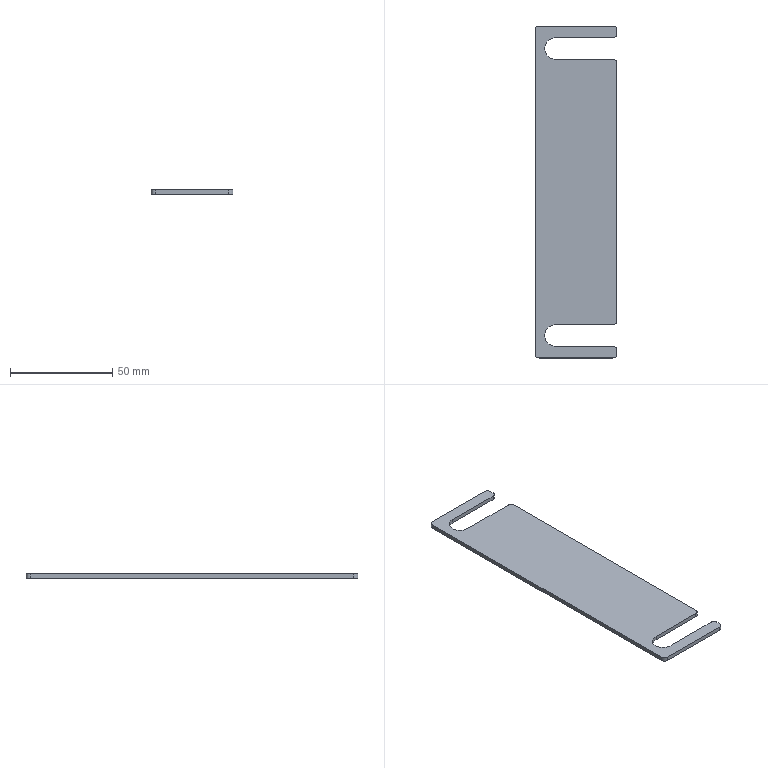Part | SolidWorks | features ICE 2, Extrusion 1, Fillet 1 | 1 solid | 22 faces | box 40 x 162 x 2 mm | volume 11517 mm3 | plane 12 | cylinder 10 | commonest cylinder face diameters 4 x8 10.5 x2
STEP:
#1=CARTESIAN_POINT('',(20.,77.25,2.));
#2=VERTEX_POINT('',#1);
#3=CARTESIAN_POINT('',(20.,79.,2.));
#4=VERTEX_POINT('',#3);
#5=CARTESIAN_POINT('',(20.,-81.,2.));
#6=DIRECTION('',(0.,1.,0.));
#7=VECTOR('',#6,1000.);
#8=LINE('',#5,#7);
#9=EDGE_CURVE('',#2,#4,#8,.T.);
#10=ORIENTED_EDGE('',*,*,#9,.F.);
#11=CARTESIAN_POINT('',(20.,77.25,0.));
#12=VERTEX_POINT('',#11);
#13=CARTESIAN_POINT('',(20.,77.25,2.));
#14=DIRECTION('',(0.,0.,-1.));
#15=VECTOR('',#14,1000.);
#16=LINE('',#13,#15);
#17=EDGE_CURVE('',#2,#12,#16,.T.);
#18=ORIENTED_EDGE('',*,*,#17,.T.);
#19=CARTESIAN_POINT('',(20.,79.,0.));
#20=VERTEX_POINT('',#19);
#21=CARTESIAN_POINT('',(20.,-81.,0.));
#22=DIRECTION('',(0.,1.,0.));
#23=VECTOR('',#22,1000.);
#24=LINE('',#21,#23);
#25=EDGE_CURVE('',#12,#20,#24,.T.);
#26=ORIENTED_EDGE('',*,*,#25,.T.);
#27=CARTESIAN_POINT('',(20.,79.,2.));
#28=DIRECTION('',(0.,0.,1.));
#29=VECTOR('',#28,1000.);
#30=LINE('',#27,#29);
#31=EDGE_CURVE('',#20,#4,#30,.T.);
#32=ORIENTED_EDGE('',*,*,#31,.T.);
#33=EDGE_LOOP('',(#10,#18,#26,#32));
#34=FACE_OUTER_BOUND('',#33,.T.);
#35=CARTESIAN_POINT('',(20.,-81.,2.));
#36=DIRECTION('',(-1.,0.,0.));
#37=DIRECTION('',(0.,0.,1.));
#38=AXIS2_PLACEMENT_3D('',#35,#36,#37);
#39=PLANE('',#38);
#40=ADVANCED_FACE('',(#34),#39,.F.);
#41=CARTESIAN_POINT('',(20.,-62.781,2.));
#42=VERTEX_POINT('',#41);
#43=CARTESIAN_POINT('',(20.,62.75,2.));
#44=VERTEX_POINT('',#43);
#45=CARTESIAN_POINT('',(20.,-81.,2.));
#46=DIRECTION('',(0.,1.,0.));
#47=VECTOR('',#46,1000.);
#48=LINE('',#45,#47);
#49=EDGE_CURVE('',#42,#44,#48,.T.);
#50=ORIENTED_EDGE('',*,*,#49,.F.);
#51=CARTESIAN_POINT('',(20.,-62.781,0.));
#52=VERTEX_POINT('',#51);
#53=CARTESIAN_POINT('',(20.,-62.781,2.));
#54=DIRECTION('',(0.,0.,-1.));
#55=VECTOR('',#54,1000.);
#56=LINE('',#53,#55);
#57=EDGE_CURVE('',#42,#52,#56,.T.);
#58=ORIENTED_EDGE('',*,*,#57,.T.);
#59=CARTESIAN_POINT('',(20.,62.75,0.));
#60=VERTEX_POINT('',#59);
#61=CARTESIAN_POINT('',(20.,-81.,0.));
#62=DIRECTION('',(0.,1.,0.));
#63=VECTOR('',#62,1000.);
#64=LINE('',#61,#63);
#65=EDGE_CURVE('',#52,#60,#64,.T.);
#66=ORIENTED_EDGE('',*,*,#65,.T.);
#67=CARTESIAN_POINT('',(20.,62.75,2.));
#68=DIRECTION('',(0.,0.,1.));
#69=VECTOR('',#68,1000.);
#70=LINE('',#67,#69);
#71=EDGE_CURVE('',#60,#44,#70,.T.);
#72=ORIENTED_EDGE('',*,*,#71,.T.);
#73=EDGE_LOOP('',(#50,#58,#66,#72));
#74=FACE_OUTER_BOUND('',#73,.T.);
#75=CARTESIAN_POINT('',(20.,-81.,2.));
#76=DIRECTION('',(-1.,0.,0.));
#77=DIRECTION('',(0.,0.,1.));
#78=AXIS2_PLACEMENT_3D('',#75,#76,#77);
#79=PLANE('',#78);
#80=ADVANCED_FACE('',(#74),#79,.F.);
#81=CARTESIAN_POINT('',(-10.,75.25,2.));
#82=VERTEX_POINT('',#81);
#83=CARTESIAN_POINT('',(-10.,75.25,0.));
#84=VERTEX_POINT('',#83);
#85=CARTESIAN_POINT('',(-10.,75.25,-1.));
#86=DIRECTION('',(0.,0.,-1.));
#87=VECTOR('',#86,1000.);
#88=LINE('',#85,#87);
#89=EDGE_CURVE('',#82,#84,#88,.T.);
#90=ORIENTED_EDGE('',*,*,#89,.F.);
#91=CARTESIAN_POINT('',(-10.,64.75,2.));
#92=VERTEX_POINT('',#91);
#93=CARTESIAN_POINT('',(-10.,70.,2.));
#94=DIRECTION('',(0.,0.,1.));
#95=DIRECTION('',(1.,0.,0.));
#96=AXIS2_PLACEMENT_3D('',#93,#94,#95);
#97=CIRCLE('',#96,5.25);
#98=EDGE_CURVE('',#82,#92,#97,.T.);
#99=ORIENTED_EDGE('',*,*,#98,.T.);
#100=CARTESIAN_POINT('',(-10.,64.75,0.));
#101=VERTEX_POINT('',#100);
#102=CARTESIAN_POINT('',(-10.,64.75,-1.));
#103=DIRECTION('',(0.,0.,-1.));
#104=VECTOR('',#103,1000.);
#105=LINE('',#102,#104);
#106=EDGE_CURVE('',#92,#101,#105,.T.);
#107=ORIENTED_EDGE('',*,*,#106,.T.);
#108=CARTESIAN_POINT('',(-10.,70.,0.));
#109=DIRECTION('',(0.,0.,1.));
#110=DIRECTION('',(1.,0.,0.));
#111=AXIS2_PLACEMENT_3D('',#108,#109,#110);
#112=CIRCLE('',#111,5.25);
#113=EDGE_CURVE('',#84,#101,#112,.T.);
#114=ORIENTED_EDGE('',*,*,#113,.F.);
#115=EDGE_LOOP('',(#90,#99,#107,#114));
#116=FACE_OUTER_BOUND('',#115,.T.);
#117=CARTESIAN_POINT('',(-10.,70.,-1.));
#118=DIRECTION('',(0.,0.,1.));
#119=DIRECTION('',(1.,0.,0.));
#120=AXIS2_PLACEMENT_3D('',#117,#118,#119);
#121=CYLINDRICAL_SURFACE('',#120,5.25);
#122=ADVANCED_FACE('',(#116),#121,.F.);
#123=CARTESIAN_POINT('',(-20.,79.,0.));
#124=VERTEX_POINT('',#123);
#125=CARTESIAN_POINT('',(-20.,-79.,0.));
#126=VERTEX_POINT('',#125);
#127=CARTESIAN_POINT('',(-20.,-81.,0.));
#128=DIRECTION('',(0.,-1.,0.));
#129=VECTOR('',#128,1000.);
#130=LINE('',#127,#129);
#131=EDGE_CURVE('',#124,#126,#130,.T.);
#132=ORIENTED_EDGE('',*,*,#131,.T.);
#133=CARTESIAN_POINT('',(-20.,-79.,2.));
#134=VERTEX_POINT('',#133);
#135=CARTESIAN_POINT('',(-20.,-79.,2.));
#136=DIRECTION('',(0.,0.,1.));
#137=VECTOR('',#136,1000.);
#138=LINE('',#135,#137);
#139=EDGE_CURVE('',#126,#134,#138,.T.);
#140=ORIENTED_EDGE('',*,*,#139,.T.);
#141=CARTESIAN_POINT('',(-20.,79.,2.));
#142=VERTEX_POINT('',#141);
#143=CARTESIAN_POINT('',(-20.,-81.,2.));
#144=DIRECTION('',(0.,-1.,0.));
#145=VECTOR('',#144,1000.);
#146=LINE('',#143,#145);
#147=EDGE_CURVE('',#142,#134,#146,.T.);
#148=ORIENTED_EDGE('',*,*,#147,.F.);
#149=CARTESIAN_POINT('',(-20.,79.,2.));
#150=DIRECTION('',(0.,0.,-1.));
#151=VECTOR('',#150,1000.);
#152=LINE('',#149,#151);
#153=EDGE_CURVE('',#142,#124,#152,.T.);
#154=ORIENTED_EDGE('',*,*,#153,.T.);
#155=EDGE_LOOP('',(#132,#140,#148,#154));
#156=FACE_OUTER_BOUND('',#155,.T.);
#157=CARTESIAN_POINT('',(-20.,-81.,2.));
#158=DIRECTION('',(1.,0.,0.));
#159=DIRECTION('',(0.,0.,-1.));
#160=AXIS2_PLACEMENT_3D('',#157,#158,#159);
#161=PLANE('',#160);
#162=ADVANCED_FACE('',(#156),#161,.F.);
#163=CARTESIAN_POINT('',(-18.,-81.,2.));
#164=VERTEX_POINT('',#163);
#165=CARTESIAN_POINT('',(18.,-81.,2.));
#166=VERTEX_POINT('',#165);
#167=CARTESIAN_POINT('',(20.,-81.,2.));
#168=DIRECTION('',(1.,0.,0.));
#169=VECTOR('',#168,1000.);
#170=LINE('',#167,#169);
#171=EDGE_CURVE('',#164,#166,#170,.T.);
#172=ORIENTED_EDGE('',*,*,#171,.F.);
#173=CARTESIAN_POINT('',(-18.,-81.,0.));
#174=VERTEX_POINT('',#173);
#175=CARTESIAN_POINT('',(-18.,-81.,2.));
#176=DIRECTION('',(0.,0.,-1.));
#177=VECTOR('',#176,1000.);
#178=LINE('',#175,#177);
#179=EDGE_CURVE('',#164,#174,#178,.T.);
#180=ORIENTED_EDGE('',*,*,#179,.T.);
#181=CARTESIAN_POINT('',(18.,-81.,0.));
#182=VERTEX_POINT('',#181);
#183=CARTESIAN_POINT('',(20.,-81.,0.));
#184=DIRECTION('',(1.,0.,0.));
#185=VECTOR('',#184,1000.);
#186=LINE('',#183,#185);
#187=EDGE_CURVE('',#174,#182,#186,.T.);
#188=ORIENTED_EDGE('',*,*,#187,.T.);
#189=CARTESIAN_POINT('',(18.,-81.,2.));
#190=DIRECTION('',(0.,0.,1.));
#191=VECTOR('',#190,1000.);
#192=LINE('',#189,#191);
#193=EDGE_CURVE('',#182,#166,#192,.T.);
#194=ORIENTED_EDGE('',*,*,#193,.T.);
#195=EDGE_LOOP('',(#172,#180,#188,#194));
#196=FACE_OUTER_BOUND('',#195,.T.);
#197=CARTESIAN_POINT('',(20.,-81.,2.));
#198=DIRECTION('',(0.,1.,0.));
#199=DIRECTION('',(0.,0.,1.));
#200=AXIS2_PLACEMENT_3D('',#197,#198,#199);
#201=PLANE('',#200);
#202=ADVANCED_FACE('',(#196),#201,.F.);
#203=CARTESIAN_POINT('',(20.,-79.,0.));
#204=VERTEX_POINT('',#203);
#205=CARTESIAN_POINT('',(20.,-77.219,0.));
#206=VERTEX_POINT('',#205);
#207=CARTESIAN_POINT('',(20.,-81.,0.));
#208=DIRECTION('',(0.,1.,0.));
#209=VECTOR('',#208,1000.);
#210=LINE('',#207,#209);
#211=EDGE_CURVE('',#204,#206,#210,.T.);
#212=ORIENTED_EDGE('',*,*,#211,.T.);
#213=CARTESIAN_POINT('',(20.,-77.219,2.));
#214=VERTEX_POINT('',#213);
#215=CARTESIAN_POINT('',(20.,-77.219,2.));
#216=DIRECTION('',(0.,0.,1.));
#217=VECTOR('',#216,1000.);
#218=LINE('',#215,#217);
#219=EDGE_CURVE('',#206,#214,#218,.T.);
#220=ORIENTED_EDGE('',*,*,#219,.T.);
#221=CARTESIAN_POINT('',(20.,-79.,2.));
#222=VERTEX_POINT('',#221);
#223=CARTESIAN_POINT('',(20.,-81.,2.));
#224=DIRECTION('',(0.,1.,0.));
#225=VECTOR('',#224,1000.);
#226=LINE('',#223,#225);
#227=EDGE_CURVE('',#222,#214,#226,.T.);
#228=ORIENTED_EDGE('',*,*,#227,.F.);
#229=CARTESIAN_POINT('',(20.,-79.,2.));
#230=DIRECTION('',(0.,0.,-1.));
#231=VECTOR('',#230,1000.);
#232=LINE('',#229,#231);
#233=EDGE_CURVE('',#222,#204,#232,.T.);
#234=ORIENTED_EDGE('',*,*,#233,.T.);
#235=EDGE_LOOP('',(#212,#220,#228,#234));
#236=FACE_OUTER_BOUND('',#235,.T.);
#237=CARTESIAN_POINT('',(20.,-81.,2.));
#238=DIRECTION('',(-1.,0.,0.));
#239=DIRECTION('',(0.,0.,1.));
#240=AXIS2_PLACEMENT_3D('',#237,#238,#239);
#241=PLANE('',#240);
#242=ADVANCED_FACE('',(#236),#241,.F.);
#243=CARTESIAN_POINT('',(18.,81.,0.));
#244=VERTEX_POINT('',#243);
#245=CARTESIAN_POINT('',(-18.,81.,0.));
#246=VERTEX_POINT('',#245);
#247=CARTESIAN_POINT('',(20.,81.,0.));
#248=DIRECTION('',(-1.,0.,0.));
#249=VECTOR('',#248,1000.);
#250=LINE('',#247,#249);
#251=EDGE_CURVE('',#244,#246,#250,.T.);
#252=ORIENTED_EDGE('',*,*,#251,.T.);
#253=CARTESIAN_POINT('',(-18.,81.,2.));
#254=VERTEX_POINT('',#253);
#255=CARTESIAN_POINT('',(-18.,81.,2.));
#256=DIRECTION('',(0.,0.,1.));
#257=VECTOR('',#256,1000.);
#258=LINE('',#255,#257);
#259=EDGE_CURVE('',#246,#254,#258,.T.);
#260=ORIENTED_EDGE('',*,*,#259,.T.);
#261=CARTESIAN_POINT('',(18.,81.,2.));
#262=VERTEX_POINT('',#261);
#263=CARTESIAN_POINT('',(20.,81.,2.));
#264=DIRECTION('',(-1.,0.,0.));
#265=VECTOR('',#264,1000.);
#266=LINE('',#263,#265);
#267=EDGE_CURVE('',#262,#254,#266,.T.);
#268=ORIENTED_EDGE('',*,*,#267,.F.);
#269=CARTESIAN_POINT('',(18.,81.,2.));
#270=DIRECTION('',(0.,0.,-1.));
#271=VECTOR('',#270,1000.);
#272=LINE('',#269,#271);
#273=EDGE_CURVE('',#262,#244,#272,.T.);
#274=ORIENTED_EDGE('',*,*,#273,.T.);
#275=EDGE_LOOP('',(#252,#260,#268,#274));
#276=FACE_OUTER_BOUND('',#275,.T.);
#277=CARTESIAN_POINT('',(20.,81.,2.));
#278=DIRECTION('',(0.,-1.,0.));
#279=DIRECTION('',(0.,0.,-1.));
#280=AXIS2_PLACEMENT_3D('',#277,#278,#279);
#281=PLANE('',#280);
#282=ADVANCED_FACE('',(#276),#281,.F.);
#283=ORIENTED_EDGE('',*,*,#227,.T.);
#284=CARTESIAN_POINT('',(18.,-75.219,2.));
#285=VERTEX_POINT('',#284);
#286=CARTESIAN_POINT('',(18.,-77.219,2.));
#287=DIRECTION('',(0.,0.,1.));
#288=DIRECTION('',(1.,0.,0.));
#289=AXIS2_PLACEMENT_3D('',#286,#287,#288);
#290=CIRCLE('',#289,2.);
#291=EDGE_CURVE('',#214,#285,#290,.T.);
#292=ORIENTED_EDGE('',*,*,#291,.T.);
#293=CARTESIAN_POINT('',(-9.434,-75.219,2.));
#294=VERTEX_POINT('',#293);
#295=CARTESIAN_POINT('',(-9.434,-75.219,2.));
#296=DIRECTION('',(1.,0.,0.));
#297=VECTOR('',#296,1000.);
#298=LINE('',#295,#297);
#299=EDGE_CURVE('',#294,#285,#298,.T.);
#300=ORIENTED_EDGE('',*,*,#299,.F.);
#301=CARTESIAN_POINT('',(-9.434,-64.781,2.));
#302=VERTEX_POINT('',#301);
#303=CARTESIAN_POINT('',(-10.,-70.,2.));
#304=DIRECTION('',(0.,0.,1.));
#305=DIRECTION('',(1.,0.,0.));
#306=AXIS2_PLACEMENT_3D('',#303,#304,#305);
#307=CIRCLE('',#306,5.25);
#308=EDGE_CURVE('',#302,#294,#307,.T.);
#309=ORIENTED_EDGE('',*,*,#308,.F.);
#310=CARTESIAN_POINT('',(18.,-64.781,2.));
#311=VERTEX_POINT('',#310);
#312=CARTESIAN_POINT('',(-9.434,-64.781,2.));
#313=DIRECTION('',(-1.,0.,0.));
#314=VECTOR('',#313,1000.);
#315=LINE('',#312,#314);
#316=EDGE_CURVE('',#311,#302,#315,.T.);
#317=ORIENTED_EDGE('',*,*,#316,.F.);
#318=CARTESIAN_POINT('',(18.,-62.781,2.));
#319=DIRECTION('',(0.,0.,1.));
#320=DIRECTION('',(1.,0.,0.));
#321=AXIS2_PLACEMENT_3D('',#318,#319,#320);
#322=CIRCLE('',#321,2.);
#323=EDGE_CURVE('',#311,#42,#322,.T.);
#324=ORIENTED_EDGE('',*,*,#323,.T.);
#325=ORIENTED_EDGE('',*,*,#49,.T.);
#326=CARTESIAN_POINT('',(18.,64.75,2.));
#327=VERTEX_POINT('',#326);
#328=CARTESIAN_POINT('',(18.,62.75,2.));
#329=DIRECTION('',(0.,0.,1.));
#330=DIRECTION('',(1.,0.,0.));
#331=AXIS2_PLACEMENT_3D('',#328,#329,#330);
#332=CIRCLE('',#331,2.);
#333=EDGE_CURVE('',#44,#327,#332,.T.);
#334=ORIENTED_EDGE('',*,*,#333,.T.);
#335=CARTESIAN_POINT('',(-10.,64.75,2.));
#336=DIRECTION('',(1.,0.,0.));
#337=VECTOR('',#336,1000.);
#338=LINE('',#335,#337);
#339=EDGE_CURVE('',#92,#327,#338,.T.);
#340=ORIENTED_EDGE('',*,*,#339,.F.);
#341=ORIENTED_EDGE('',*,*,#98,.F.);
#342=CARTESIAN_POINT('',(18.,75.25,2.));
#343=VERTEX_POINT('',#342);
#344=CARTESIAN_POINT('',(-10.,75.25,2.));
#345=DIRECTION('',(-1.,0.,0.));
#346=VECTOR('',#345,1000.);
#347=LINE('',#344,#346);
#348=EDGE_CURVE('',#343,#82,#347,.T.);
#349=ORIENTED_EDGE('',*,*,#348,.F.);
#350=CARTESIAN_POINT('',(18.,77.25,2.));
#351=DIRECTION('',(0.,0.,1.));
#352=DIRECTION('',(1.,0.,0.));
#353=AXIS2_PLACEMENT_3D('',#350,#351,#352);
#354=CIRCLE('',#353,2.);
#355=EDGE_CURVE('',#343,#2,#354,.T.);
#356=ORIENTED_EDGE('',*,*,#355,.T.);
#357=ORIENTED_EDGE('',*,*,#9,.T.);
#358=CARTESIAN_POINT('',(18.,79.,2.));
#359=DIRECTION('',(0.,0.,1.));
#360=DIRECTION('',(1.,0.,0.));
#361=AXIS2_PLACEMENT_3D('',#358,#359,#360);
#362=CIRCLE('',#361,2.);
#363=EDGE_CURVE('',#4,#262,#362,.T.);
#364=ORIENTED_EDGE('',*,*,#363,.T.);
#365=ORIENTED_EDGE('',*,*,#267,.T.);
#366=CARTESIAN_POINT('',(-18.,79.,2.));
#367=DIRECTION('',(0.,0.,1.));
#368=DIRECTION('',(1.,0.,0.));
#369=AXIS2_PLACEMENT_3D('',#366,#367,#368);
#370=CIRCLE('',#369,2.);
#371=EDGE_CURVE('',#254,#142,#370,.T.);
#372=ORIENTED_EDGE('',*,*,#371,.T.);
#373=ORIENTED_EDGE('',*,*,#147,.T.);
#374=CARTESIAN_POINT('',(-18.,-79.,2.));
#375=DIRECTION('',(0.,0.,1.));
#376=DIRECTION('',(1.,0.,0.));
#377=AXIS2_PLACEMENT_3D('',#374,#375,#376);
#378=CIRCLE('',#377,2.);
#379=EDGE_CURVE('',#134,#164,#378,.T.);
#380=ORIENTED_EDGE('',*,*,#379,.T.);
#381=ORIENTED_EDGE('',*,*,#171,.T.);
#382=CARTESIAN_POINT('',(18.,-79.,2.));
#383=DIRECTION('',(0.,0.,1.));
#384=DIRECTION('',(1.,0.,0.));
#385=AXIS2_PLACEMENT_3D('',#382,#383,#384);
#386=CIRCLE('',#385,2.);
#387=EDGE_CURVE('',#166,#222,#386,.T.);
#388=ORIENTED_EDGE('',*,*,#387,.T.);
#389=EDGE_LOOP('',(#283,#292,#300,#309,#317,#324,#325,#334,#340,#341,#349,#356,#357,#364,#365,#372,#373,#380,#381,#388));
#390=FACE_OUTER_BOUND('',#389,.T.);
#391=CARTESIAN_POINT('',(0.,0.,2.));
#392=DIRECTION('',(0.,0.,1.));
#393=DIRECTION('',(1.,0.,0.));
#394=AXIS2_PLACEMENT_3D('',#391,#392,#393);
#395=PLANE('',#394);
#396=ADVANCED_FACE('',(#390),#395,.T.);
#397=CARTESIAN_POINT('',(-9.434,-75.219,0.));
#398=VERTEX_POINT('',#397);
#399=CARTESIAN_POINT('',(18.,-75.219,0.));
#400=VERTEX_POINT('',#399);
#401=CARTESIAN_POINT('',(0.,-75.219,0.));
#402=DIRECTION('',(1.,0.,0.));
#403=VECTOR('',#402,1000.);
#404=LINE('',#401,#403);
#405=EDGE_CURVE('',#398,#400,#404,.T.);
#406=ORIENTED_EDGE('',*,*,#405,.T.);
#407=CARTESIAN_POINT('',(18.,-77.219,0.));
#408=DIRECTION('',(0.,0.,-1.));
#409=DIRECTION('',(1.,0.,0.));
#410=AXIS2_PLACEMENT_3D('',#407,#408,#409);
#411=CIRCLE('',#410,2.);
#412=EDGE_CURVE('',#400,#206,#411,.T.);
#413=ORIENTED_EDGE('',*,*,#412,.T.);
#414=ORIENTED_EDGE('',*,*,#211,.F.);
#415=CARTESIAN_POINT('',(18.,-79.,0.));
#416=DIRECTION('',(0.,0.,-1.));
#417=DIRECTION('',(1.,0.,0.));
#418=AXIS2_PLACEMENT_3D('',#415,#416,#417);
#419=CIRCLE('',#418,2.);
#420=EDGE_CURVE('',#204,#182,#419,.T.);
#421=ORIENTED_EDGE('',*,*,#420,.T.);
#422=ORIENTED_EDGE('',*,*,#187,.F.);
#423=CARTESIAN_POINT('',(-18.,-79.,0.));
#424=DIRECTION('',(0.,0.,-1.));
#425=DIRECTION('',(1.,0.,0.));
#426=AXIS2_PLACEMENT_3D('',#423,#424,#425);
#427=CIRCLE('',#426,2.);
#428=EDGE_CURVE('',#174,#126,#427,.T.);
#429=ORIENTED_EDGE('',*,*,#428,.T.);
#430=ORIENTED_EDGE('',*,*,#131,.F.);
#431=CARTESIAN_POINT('',(-18.,79.,0.));
#432=DIRECTION('',(0.,0.,-1.));
#433=DIRECTION('',(1.,0.,0.));
#434=AXIS2_PLACEMENT_3D('',#431,#432,#433);
#435=CIRCLE('',#434,2.);
#436=EDGE_CURVE('',#124,#246,#435,.T.);
#437=ORIENTED_EDGE('',*,*,#436,.T.);
#438=ORIENTED_EDGE('',*,*,#251,.F.);
#439=CARTESIAN_POINT('',(18.,79.,0.));
#440=DIRECTION('',(0.,0.,-1.));
#441=DIRECTION('',(1.,0.,0.));
#442=AXIS2_PLACEMENT_3D('',#439,#440,#441);
#443=CIRCLE('',#442,2.);
#444=EDGE_CURVE('',#244,#20,#443,.T.);
#445=ORIENTED_EDGE('',*,*,#444,.T.);
#446=ORIENTED_EDGE('',*,*,#25,.F.);
#447=CARTESIAN_POINT('',(18.,75.25,0.));
#448=VERTEX_POINT('',#447);
#449=CARTESIAN_POINT('',(18.,77.25,0.));
#450=DIRECTION('',(0.,0.,-1.));
#451=DIRECTION('',(1.,0.,0.));
#452=AXIS2_PLACEMENT_3D('',#449,#450,#451);
#453=CIRCLE('',#452,2.);
#454=EDGE_CURVE('',#12,#448,#453,.T.);
#455=ORIENTED_EDGE('',*,*,#454,.T.);
#456=CARTESIAN_POINT('',(0.,75.25,0.));
#457=DIRECTION('',(-1.,0.,0.));
#458=VECTOR('',#457,1000.);
#459=LINE('',#456,#458);
#460=EDGE_CURVE('',#448,#84,#459,.T.);
#461=ORIENTED_EDGE('',*,*,#460,.T.);
#462=ORIENTED_EDGE('',*,*,#113,.T.);
#463=CARTESIAN_POINT('',(18.,64.75,0.));
#464=VERTEX_POINT('',#463);
#465=CARTESIAN_POINT('',(0.,64.75,0.));
#466=DIRECTION('',(1.,0.,0.));
#467=VECTOR('',#466,1000.);
#468=LINE('',#465,#467);
#469=EDGE_CURVE('',#101,#464,#468,.T.);
#470=ORIENTED_EDGE('',*,*,#469,.T.);
#471=CARTESIAN_POINT('',(18.,62.75,0.));
#472=DIRECTION('',(0.,0.,-1.));
#473=DIRECTION('',(1.,0.,0.));
#474=AXIS2_PLACEMENT_3D('',#471,#472,#473);
#475=CIRCLE('',#474,2.);
#476=EDGE_CURVE('',#464,#60,#475,.T.);
#477=ORIENTED_EDGE('',*,*,#476,.T.);
#478=ORIENTED_EDGE('',*,*,#65,.F.);
#479=CARTESIAN_POINT('',(18.,-64.781,0.));
#480=VERTEX_POINT('',#479);
#481=CARTESIAN_POINT('',(18.,-62.781,0.));
#482=DIRECTION('',(0.,0.,-1.));
#483=DIRECTION('',(1.,0.,0.));
#484=AXIS2_PLACEMENT_3D('',#481,#482,#483);
#485=CIRCLE('',#484,2.);
#486=EDGE_CURVE('',#52,#480,#485,.T.);
#487=ORIENTED_EDGE('',*,*,#486,.T.);
#488=CARTESIAN_POINT('',(-9.434,-64.781,0.));
#489=VERTEX_POINT('',#488);
#490=CARTESIAN_POINT('',(0.,-64.781,0.));
#491=DIRECTION('',(-1.,0.,0.));
#492=VECTOR('',#491,1000.);
#493=LINE('',#490,#492);
#494=EDGE_CURVE('',#480,#489,#493,.T.);
#495=ORIENTED_EDGE('',*,*,#494,.T.);
#496=CARTESIAN_POINT('',(-10.,-70.,0.));
#497=DIRECTION('',(0.,0.,1.));
#498=DIRECTION('',(1.,0.,0.));
#499=AXIS2_PLACEMENT_3D('',#496,#497,#498);
#500=CIRCLE('',#499,5.25);
#501=EDGE_CURVE('',#489,#398,#500,.T.);
#502=ORIENTED_EDGE('',*,*,#501,.T.);
#503=EDGE_LOOP('',(#406,#413,#414,#421,#422,#429,#430,#437,#438,#445,#446,#455,#461,#462,#470,#477,#478,#487,#495,#502));
#504=FACE_OUTER_BOUND('',#503,.T.);
#505=CARTESIAN_POINT('',(0.,0.,0.));
#506=DIRECTION('',(0.,0.,1.));
#507=DIRECTION('',(1.,0.,0.));
#508=AXIS2_PLACEMENT_3D('',#505,#506,#507);
#509=PLANE('',#508);
#510=ADVANCED_FACE('',(#504),#509,.F.);
#511=ORIENTED_EDGE('',*,*,#501,.F.);
#512=CARTESIAN_POINT('',(-9.434,-64.781,-1.));
#513=DIRECTION('',(0.,0.,1.));
#514=VECTOR('',#513,1000.);
#515=LINE('',#512,#514);
#516=EDGE_CURVE('',#489,#302,#515,.T.);
#517=ORIENTED_EDGE('',*,*,#516,.T.);
#518=ORIENTED_EDGE('',*,*,#308,.T.);
#519=CARTESIAN_POINT('',(-9.434,-75.219,-1.));
#520=DIRECTION('',(0.,0.,-1.));
#521=VECTOR('',#520,1000.);
#522=LINE('',#519,#521);
#523=EDGE_CURVE('',#294,#398,#522,.T.);
#524=ORIENTED_EDGE('',*,*,#523,.T.);
#525=EDGE_LOOP('',(#511,#517,#518,#524));
#526=FACE_OUTER_BOUND('',#525,.T.);
#527=CARTESIAN_POINT('',(-10.,-70.,-1.));
#528=DIRECTION('',(0.,0.,1.));
#529=DIRECTION('',(1.,0.,0.));
#530=AXIS2_PLACEMENT_3D('',#527,#528,#529);
#531=CYLINDRICAL_SURFACE('',#530,5.25);
#532=ADVANCED_FACE('',(#526),#531,.F.);
#533=ORIENTED_EDGE('',*,*,#339,.T.);
#534=CARTESIAN_POINT('',(18.,64.75,-8.));
#535=DIRECTION('',(0.,0.,-1.));
#536=VECTOR('',#535,1000.);
#537=LINE('',#534,#536);
#538=EDGE_CURVE('',#327,#464,#537,.T.);
#539=ORIENTED_EDGE('',*,*,#538,.T.);
#540=ORIENTED_EDGE('',*,*,#469,.F.);
#541=ORIENTED_EDGE('',*,*,#106,.F.);
#542=EDGE_LOOP('',(#533,#539,#540,#541));
#543=FACE_OUTER_BOUND('',#542,.T.);
#544=CARTESIAN_POINT('',(-10.,64.75,-8.));
#545=DIRECTION('',(0.,-1.,0.));
#546=DIRECTION('',(0.,0.,-1.));
#547=AXIS2_PLACEMENT_3D('',#544,#545,#546);
#548=PLANE('',#547);
#549=ADVANCED_FACE('',(#543),#548,.F.);
#550=ORIENTED_EDGE('',*,*,#460,.F.);
#551=CARTESIAN_POINT('',(18.,75.25,-8.));
#552=DIRECTION('',(0.,0.,1.));
#553=VECTOR('',#552,1000.);
#554=LINE('',#551,#553);
#555=EDGE_CURVE('',#448,#343,#554,.T.);
#556=ORIENTED_EDGE('',*,*,#555,.T.);
#557=ORIENTED_EDGE('',*,*,#348,.T.);
#558=ORIENTED_EDGE('',*,*,#89,.T.);
#559=EDGE_LOOP('',(#550,#556,#557,#558));
#560=FACE_OUTER_BOUND('',#559,.T.);
#561=CARTESIAN_POINT('',(-10.,75.25,-8.));
#562=DIRECTION('',(0.,1.,0.));
#563=DIRECTION('',(-1.,0.,0.));
#564=AXIS2_PLACEMENT_3D('',#561,#562,#563);
#565=PLANE('',#564);
#566=ADVANCED_FACE('',(#560),#565,.F.);
#567=ORIENTED_EDGE('',*,*,#299,.T.);
#568=CARTESIAN_POINT('',(18.,-75.219,-8.));
#569=DIRECTION('',(0.,0.,-1.));
#570=VECTOR('',#569,1000.);
#571=LINE('',#568,#570);
#572=EDGE_CURVE('',#285,#400,#571,.T.);
#573=ORIENTED_EDGE('',*,*,#572,.T.);
#574=ORIENTED_EDGE('',*,*,#405,.F.);
#575=ORIENTED_EDGE('',*,*,#523,.F.);
#576=EDGE_LOOP('',(#567,#573,#574,#575));
#577=FACE_OUTER_BOUND('',#576,.T.);
#578=CARTESIAN_POINT('',(-9.434,-75.219,-8.));
#579=DIRECTION('',(0.,-1.,0.));
#580=DIRECTION('',(0.,0.,-1.));
#581=AXIS2_PLACEMENT_3D('',#578,#579,#580);
#582=PLANE('',#581);
#583=ADVANCED_FACE('',(#577),#582,.F.);
#584=ORIENTED_EDGE('',*,*,#494,.F.);
#585=CARTESIAN_POINT('',(18.,-64.781,-8.));
#586=DIRECTION('',(0.,0.,1.));
#587=VECTOR('',#586,1000.);
#588=LINE('',#585,#587);
#589=EDGE_CURVE('',#480,#311,#588,.T.);
#590=ORIENTED_EDGE('',*,*,#589,.T.);
#591=ORIENTED_EDGE('',*,*,#316,.T.);
#592=ORIENTED_EDGE('',*,*,#516,.F.);
#593=EDGE_LOOP('',(#584,#590,#591,#592));
#594=FACE_OUTER_BOUND('',#593,.T.);
#595=CARTESIAN_POINT('',(-9.434,-64.781,-8.));
#596=DIRECTION('',(0.,1.,0.));
#597=DIRECTION('',(0.,0.,1.));
#598=AXIS2_PLACEMENT_3D('',#595,#596,#597);
#599=PLANE('',#598);
#600=ADVANCED_FACE('',(#594),#599,.F.);
#601=ORIENTED_EDGE('',*,*,#412,.F.);
#602=ORIENTED_EDGE('',*,*,#572,.F.);
#603=ORIENTED_EDGE('',*,*,#291,.F.);
#604=ORIENTED_EDGE('',*,*,#219,.F.);
#605=EDGE_LOOP('',(#601,#602,#603,#604));
#606=FACE_OUTER_BOUND('',#605,.T.);
#607=CARTESIAN_POINT('',(18.,-77.219,2.));
#608=DIRECTION('',(0.,0.,1.));
#609=DIRECTION('',(1.,0.,0.));
#610=AXIS2_PLACEMENT_3D('',#607,#608,#609);
#611=CYLINDRICAL_SURFACE('',#610,2.);
#612=ADVANCED_FACE('',(#606),#611,.T.);
#613=ORIENTED_EDGE('',*,*,#486,.F.);
#614=ORIENTED_EDGE('',*,*,#57,.F.);
#615=ORIENTED_EDGE('',*,*,#323,.F.);
#616=ORIENTED_EDGE('',*,*,#589,.F.);
#617=EDGE_LOOP('',(#613,#614,#615,#616));
#618=FACE_OUTER_BOUND('',#617,.T.);
#619=CARTESIAN_POINT('',(18.,-62.781,-8.));
#620=DIRECTION('',(0.,0.,1.));
#621=DIRECTION('',(1.,0.,0.));
#622=AXIS2_PLACEMENT_3D('',#619,#620,#621);
#623=CYLINDRICAL_SURFACE('',#622,2.);
#624=ADVANCED_FACE('',(#618),#623,.T.);
#625=ORIENTED_EDGE('',*,*,#476,.F.);
#626=ORIENTED_EDGE('',*,*,#538,.F.);
#627=ORIENTED_EDGE('',*,*,#333,.F.);
#628=ORIENTED_EDGE('',*,*,#71,.F.);
#629=EDGE_LOOP('',(#625,#626,#627,#628));
#630=FACE_OUTER_BOUND('',#629,.T.);
#631=CARTESIAN_POINT('',(18.,62.75,2.));
#632=DIRECTION('',(0.,0.,1.));
#633=DIRECTION('',(1.,0.,0.));
#634=AXIS2_PLACEMENT_3D('',#631,#632,#633);
#635=CYLINDRICAL_SURFACE('',#634,2.);
#636=ADVANCED_FACE('',(#630),#635,.T.);
#637=ORIENTED_EDGE('',*,*,#454,.F.);
#638=ORIENTED_EDGE('',*,*,#17,.F.);
#639=ORIENTED_EDGE('',*,*,#355,.F.);
#640=ORIENTED_EDGE('',*,*,#555,.F.);
#641=EDGE_LOOP('',(#637,#638,#639,#640));
#642=FACE_OUTER_BOUND('',#641,.T.);
#643=CARTESIAN_POINT('',(18.,77.25,-8.));
#644=DIRECTION('',(0.,0.,1.));
#645=DIRECTION('',(1.,0.,0.));
#646=AXIS2_PLACEMENT_3D('',#643,#644,#645);
#647=CYLINDRICAL_SURFACE('',#646,2.);
#648=ADVANCED_FACE('',(#642),#647,.T.);
#649=ORIENTED_EDGE('',*,*,#379,.F.);
#650=ORIENTED_EDGE('',*,*,#139,.F.);
#651=ORIENTED_EDGE('',*,*,#428,.F.);
#652=ORIENTED_EDGE('',*,*,#179,.F.);
#653=EDGE_LOOP('',(#649,#650,#651,#652));
#654=FACE_OUTER_BOUND('',#653,.T.);
#655=CARTESIAN_POINT('',(-18.,-79.,2.));
#656=DIRECTION('',(0.,0.,-1.));
#657=DIRECTION('',(-1.,0.,0.));
#658=AXIS2_PLACEMENT_3D('',#655,#656,#657);
#659=CYLINDRICAL_SURFACE('',#658,2.);
#660=ADVANCED_FACE('',(#654),#659,.T.);
#661=ORIENTED_EDGE('',*,*,#371,.F.);
#662=ORIENTED_EDGE('',*,*,#259,.F.);
#663=ORIENTED_EDGE('',*,*,#436,.F.);
#664=ORIENTED_EDGE('',*,*,#153,.F.);
#665=EDGE_LOOP('',(#661,#662,#663,#664));
#666=FACE_OUTER_BOUND('',#665,.T.);
#667=CARTESIAN_POINT('',(-18.,79.,2.));
#668=DIRECTION('',(0.,0.,-1.));
#669=DIRECTION('',(-1.,0.,0.));
#670=AXIS2_PLACEMENT_3D('',#667,#668,#669);
#671=CYLINDRICAL_SURFACE('',#670,2.);
#672=ADVANCED_FACE('',(#666),#671,.T.);
#673=ORIENTED_EDGE('',*,*,#387,.F.);
#674=ORIENTED_EDGE('',*,*,#193,.F.);
#675=ORIENTED_EDGE('',*,*,#420,.F.);
#676=ORIENTED_EDGE('',*,*,#233,.F.);
#677=EDGE_LOOP('',(#673,#674,#675,#676));
#678=FACE_OUTER_BOUND('',#677,.T.);
#679=CARTESIAN_POINT('',(18.,-79.,2.));
#680=DIRECTION('',(0.,0.,-1.));
#681=DIRECTION('',(-1.,0.,0.));
#682=AXIS2_PLACEMENT_3D('',#679,#680,#681);
#683=CYLINDRICAL_SURFACE('',#682,2.);
#684=ADVANCED_FACE('',(#678),#683,.T.);
#685=ORIENTED_EDGE('',*,*,#363,.F.);
#686=ORIENTED_EDGE('',*,*,#31,.F.);
#687=ORIENTED_EDGE('',*,*,#444,.F.);
#688=ORIENTED_EDGE('',*,*,#273,.F.);
#689=EDGE_LOOP('',(#685,#686,#687,#688));
#690=FACE_OUTER_BOUND('',#689,.T.);
#691=CARTESIAN_POINT('',(18.,79.,2.));
#692=DIRECTION('',(0.,0.,-1.));
#693=DIRECTION('',(-1.,0.,0.));
#694=AXIS2_PLACEMENT_3D('',#691,#692,#693);
#695=CYLINDRICAL_SURFACE('',#694,2.);
#696=ADVANCED_FACE('',(#690),#695,.T.);
#697=CLOSED_SHELL('',(#40,#80,#122,#162,#202,#242,#282,#396,#510,#532,#549,#566,#583,#600,#612,#624,#636,#648,#660,#672,#684,#696));
#698=MANIFOLD_SOLID_BREP('',#697);
#699=CARTESIAN_POINT('',(0.,0.,0.));
#700=DIRECTION('',(0.,0.,1.));
#701=DIRECTION('',(1.,0.,0.));
#702=AXIS2_PLACEMENT_3D('',#699,#700,#701);
#703=(LENGTH_UNIT()NAMED_UNIT(*)SI_UNIT(.MILLI.,.METRE.));
#704=UNCERTAINTY_MEASURE_WITH_UNIT(LENGTH_MEASURE(0.00001),#703,'','');
#705=(NAMED_UNIT(*)PLANE_ANGLE_UNIT()SI_UNIT($,.RADIAN.));
#706=(NAMED_UNIT(*)SI_UNIT($,.STERADIAN.)SOLID_ANGLE_UNIT());
#707=(GEOMETRIC_REPRESENTATION_CONTEXT(3)GLOBAL_UNCERTAINTY_ASSIGNED_CONTEXT((#704))GLOBAL_UNIT_ASSIGNED_CONTEXT((#703,#705,#706))REPRESENTATION_CONTEXT('',''));
#708=ADVANCED_BREP_SHAPE_REPRESENTATION('',(#698,#702),#707);